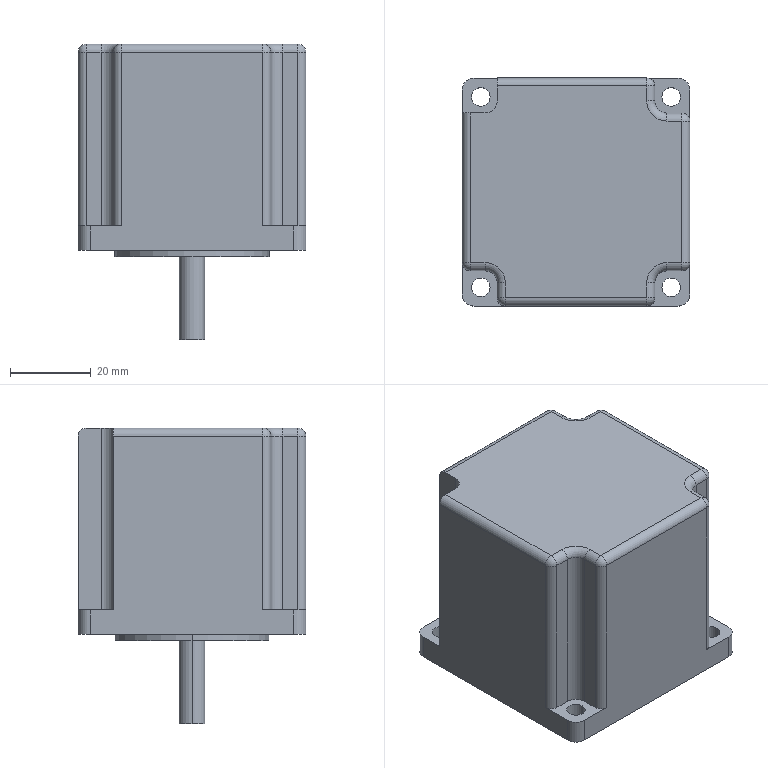Part | STEP file | QA-SM57-51C | 1 solid | 65 faces | box 56.4 x 56.4 x 73.2 mm | volume 150583 mm3 | cylinder 36 | plane 20 | sphere 6 | torus 3 | commonest cylinder face diameters 4 x16 4.6 x8 6 x8 6.35 x2 38.1 x2